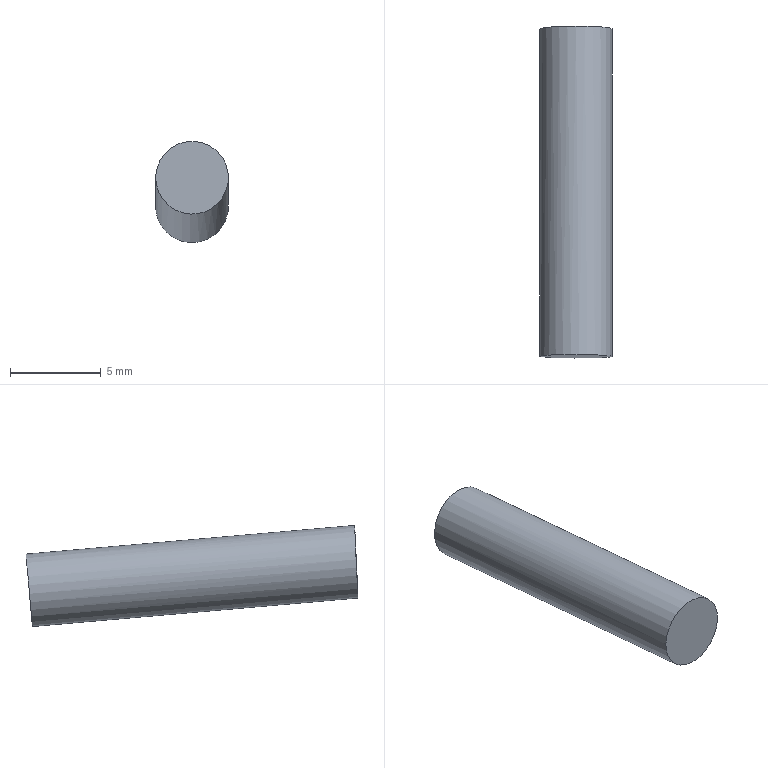Part | NX | features solid 2 | 1 solid | 3 faces | box 4 x 18.244 x 5.565 mm | volume 226.791 mm3 | plane 2 | cylinder 1 | commonest cylinder face diameters 4 x1
STEP:
#1=CARTESIAN_POINT('',(156.524,-29.244,-60.952));
#2=VERTEX_POINT('',#1);
#3=CARTESIAN_POINT('',(156.524,-29.418,-62.944));
#4=DIRECTION('',(0.,-0.9962,0.08716));
#5=DIRECTION('',(0.,0.08716,0.9962));
#6=AXIS2_PLACEMENT_3D('',#3,#4,#5);
#7=CIRCLE('',#6,2.);
#8=EDGE_CURVE('',#2,#2,#7,.T.);
#9=ORIENTED_EDGE('',*,*,#8,.F.);
#10=EDGE_LOOP('',(#9));
#11=FACE_BOUND('',#10,.T.);
#12=CARTESIAN_POINT('',(156.524,-29.418,-62.944));
#13=DIRECTION('',(0.,0.9962,-0.08716));
#14=DIRECTION('',(0.,-0.08716,-0.9962));
#15=AXIS2_PLACEMENT_3D('',#12,#13,#14);
#16=PLANE('',#15);
#17=ADVANCED_FACE('',(#11),#16,.T.);
#18=CARTESIAN_POINT('',(156.43,-47.488,-63.369));
#19=VERTEX_POINT('',#18);
#20=CARTESIAN_POINT('',(156.524,-47.397,-61.371));
#21=DIRECTION('',(0.001957,0.999,-0.04546));
#22=DIRECTION('',(-0.04675,-0.04532,-0.9979));
#23=AXIS2_PLACEMENT_3D('',#20,#21,#22);
#24=ELLIPSE('',#23,2.002,2.);
#25=EDGE_CURVE('',#19,#19,#24,.T.);
#26=ORIENTED_EDGE('',*,*,#25,.F.);
#27=EDGE_LOOP('',(#26));
#28=FACE_BOUND('',#27,.T.);
#29=CARTESIAN_POINT('',(128.811,-48.589,-88.763));
#30=DIRECTION('',(0.001957,0.999,-0.04546));
#31=DIRECTION('',(0.06617,0.04523,0.9968));
#32=AXIS2_PLACEMENT_3D('',#29,#30,#31);
#33=PLANE('',#32);
#34=ADVANCED_FACE('',(#28),#33,.F.);
#35=ORIENTED_EDGE('',*,*,#8,.T.);
#36=EDGE_LOOP('',(#35));
#37=FACE_BOUND('',#36,.T.);
#38=ORIENTED_EDGE('',*,*,#25,.T.);
#39=EDGE_LOOP('',(#38));
#40=FACE_BOUND('',#39,.T.);
#41=CARTESIAN_POINT('',(156.524,-49.342,-61.201));
#42=DIRECTION('',(0.,0.9962,-0.08716));
#43=DIRECTION('',(0.,-0.08716,-0.9962));
#44=AXIS2_PLACEMENT_3D('',#41,#42,#43);
#45=CYLINDRICAL_SURFACE('',#44,2.);
#46=ADVANCED_FACE('',(#37,#40),#45,.T.);
#47=CLOSED_SHELL('',(#17,#34,#46));
#48=MANIFOLD_SOLID_BREP('',#47);
#49=(LENGTH_UNIT()NAMED_UNIT(*)SI_UNIT(.MILLI.,.METRE.));
#50=UNCERTAINTY_MEASURE_WITH_UNIT(LENGTH_MEASURE(0.00001),#49,'','');
#51=(NAMED_UNIT(*)PLANE_ANGLE_UNIT()SI_UNIT($,.RADIAN.));
#52=(NAMED_UNIT(*)SI_UNIT($,.STERADIAN.)SOLID_ANGLE_UNIT());
#53=(GEOMETRIC_REPRESENTATION_CONTEXT(3)GLOBAL_UNCERTAINTY_ASSIGNED_CONTEXT((#50))GLOBAL_UNIT_ASSIGNED_CONTEXT((#49,#51,#52))REPRESENTATION_CONTEXT('',''));
#54=ADVANCED_BREP_SHAPE_REPRESENTATION('',(#48),#53);